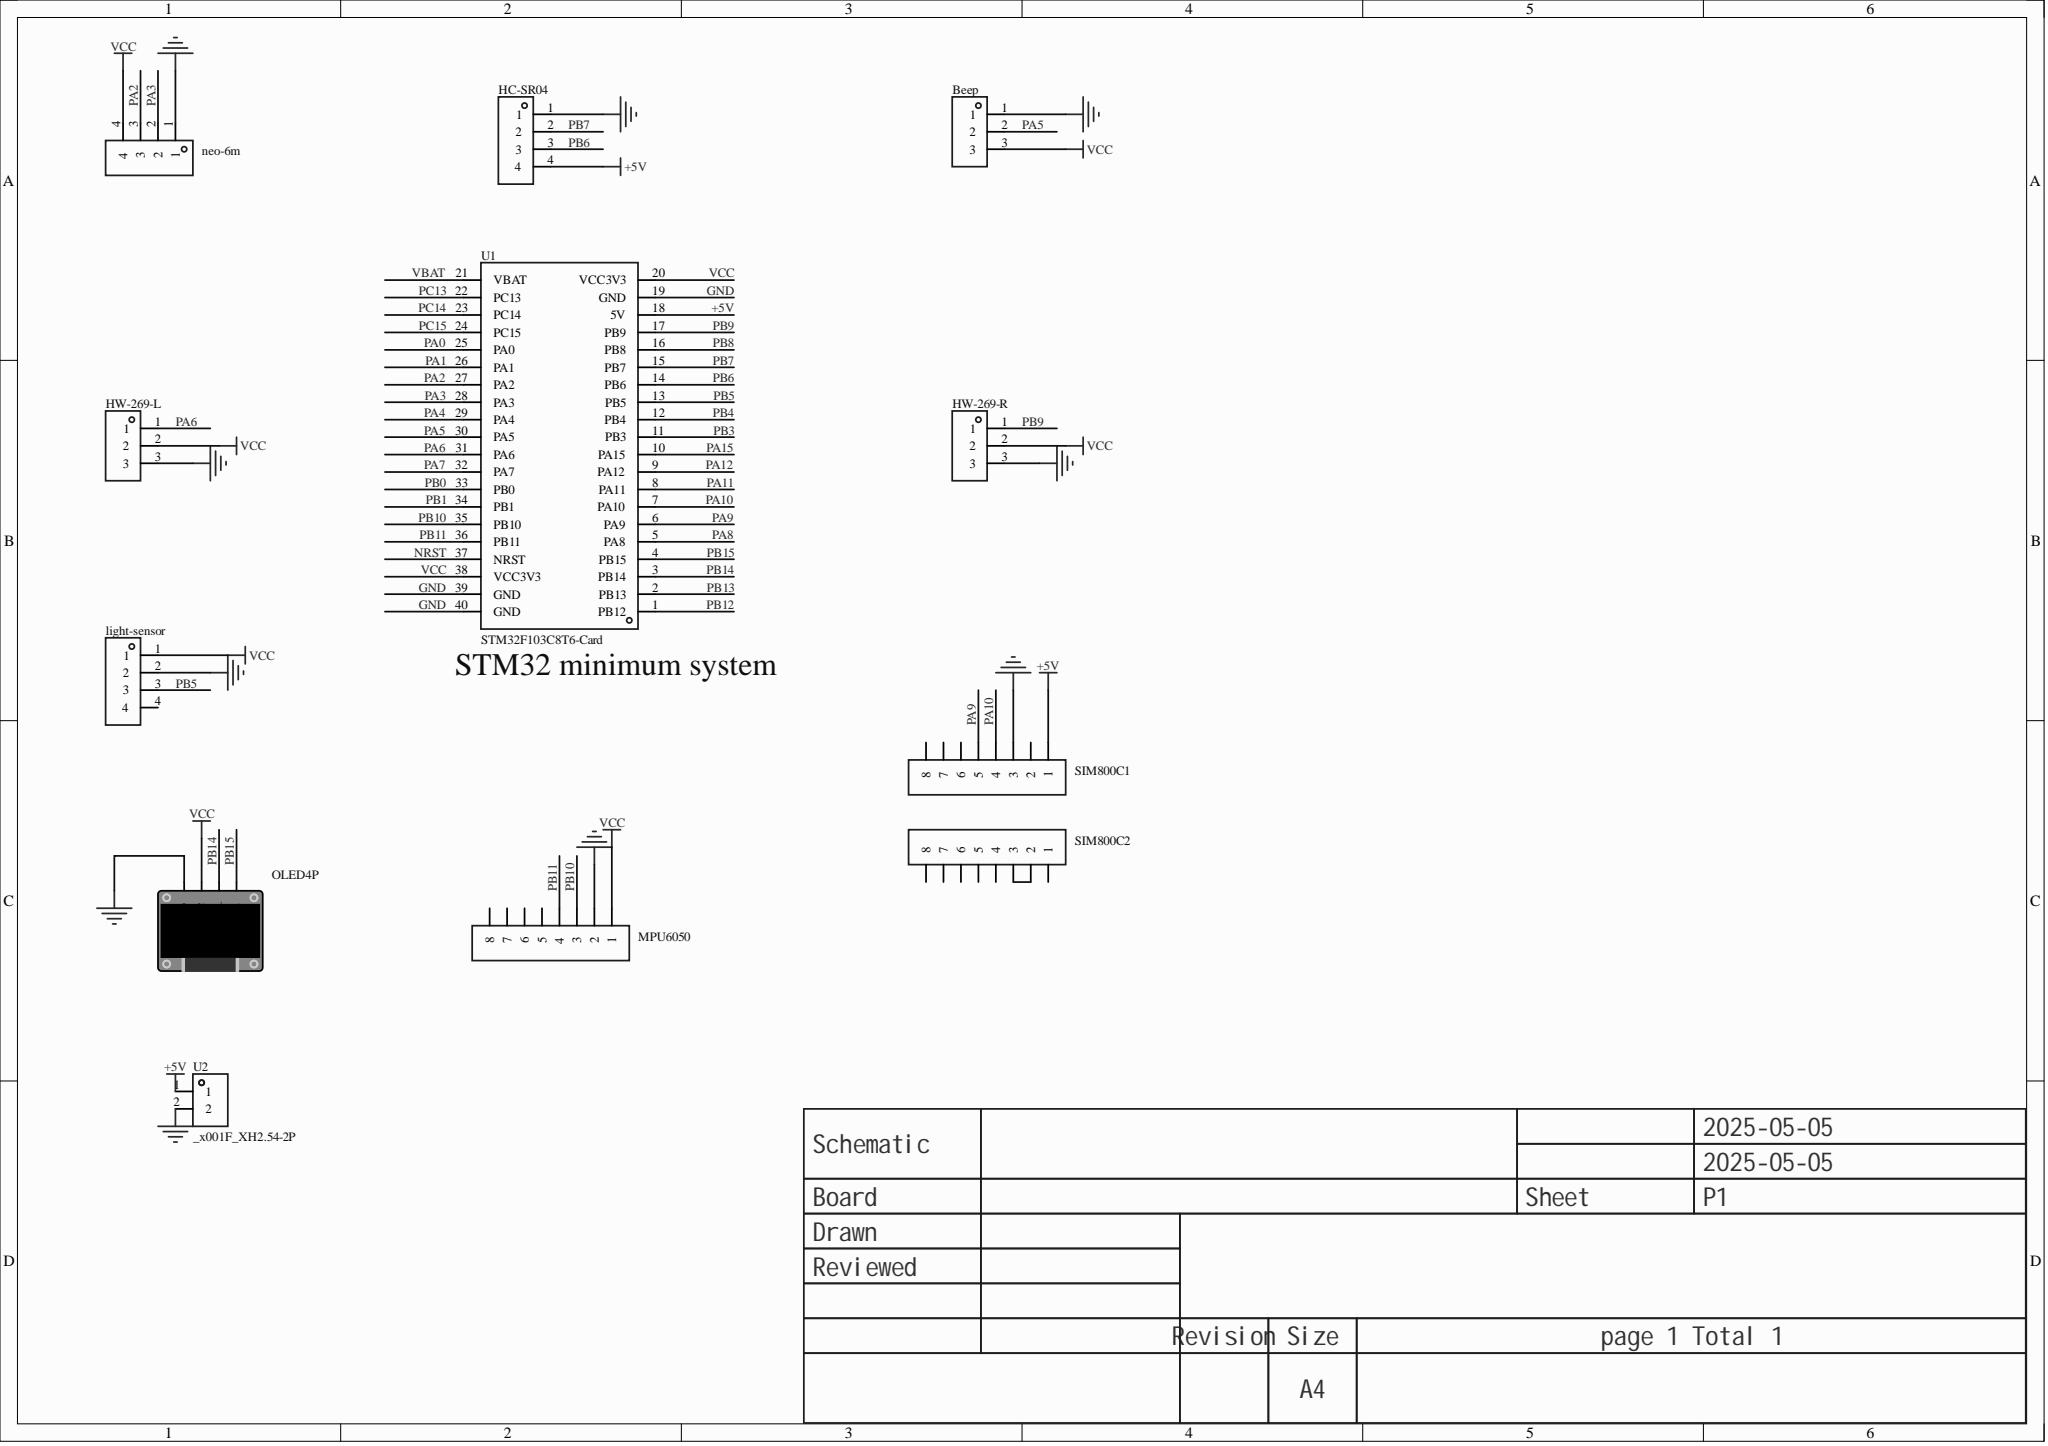Circuit board | Altium Designer | 12 parts | 18 nets
Bill of materials:
Comment,Description,Designator,Footprint,LibRef,Quantity
"","","Beep, HW-269-L, HW-269-R","HDR-TH_3P-P2.54-V-F","HDR-F_2.54_1x3P","3"
"","","HC-SR04, light-sensor, neo-6m","HDR-TH_4P-P2.54-V-F","HDR-F_2.54_1x4P","3"
"","","MPU6050, SIM800C1, SIM800C2","HDR-TH_8P-P2.54-V-F-1","HDR-F_2.54_1x8P","3"
"","","OLED4P","0.96OLED_4P","0.96OLED模块_4P","1"
"STM32F103C8T6-Card","","U1","CONN-TH_L53.3-W22.9_STM32F103C8T6-CARD","STM32F103C8T6-Card","1"
"_x001F_XH2.54-2P","","U2","CONN-TH_2P-P2.54-V","_x001F_XH2.54-2P","1"
Netlist (Protel format):
[
Beep
HDR-TH_3P-P2.54-V-F




]
[
HC-SR04
HDR-TH_4P-P2.54-V-F




]
[
HW-269-L
HDR-TH_3P-P2.54-V-F




]
[
HW-269-R
HDR-TH_3P-P2.54-V-F




]
[
light-sensor
HDR-TH_4P-P2.54-V-F




]
[
MPU6050
HDR-TH_8P-P2.54-V-F-1




]
[
neo-6m
HDR-TH_4P-P2.54-V-F




]
[
OLED4P
0.96OLED_4P




]
[
SIM800C1
HDR-TH_8P-P2.54-V-F-1




]
[
SIM800C2
HDR-TH_8P-P2.54-V-F-1




]
[
U1
CONN-TH_L53.3-W22.9_STM32F103C8T6-CARD
STM32F103C8T6-Card



]
[
U2
CONN-TH_2P-P2.54-V
_x001F_XH2.54-2P



]
(
VCC
Beep-3
HW-269-L-2
HW-269-R-2
light-sensor-1
MPU6050-1
neo-6m-4
OLED4P-2
U1-20
U1-38
)
(
PB15
OLED4P-4
U1-4
)
(
PB14
OLED4P-3
U1-3
)
(
PB11
MPU6050-4
U1-36
)
(
PB10
MPU6050-3
U1-35
)
(
PB9
HW-269-R-1
U1-17
)
(
PB7
HC-SR04-2
U1-15
)
(
PB6
HC-SR04-3
U1-14
)
(
PB5
light-sensor-3
U1-13
)
(
PA10
SIM800C1-4
U1-7
)
(
PA9
SIM800C1-5
U1-6
)
(
PA6
HW-269-L-1
U1-31
)
(
PA5
Beep-2
U1-30
)
(
PA3
neo-6m-2
U1-28
)
(
PA2
neo-6m-3
U1-27
)
(
NetSIM800C2_2
SIM800C2-2
SIM800C2-3
)
(
GND
Beep-1
HC-SR04-1
HW-269-L-3
HW-269-R-3
light-sensor-2
MPU6050-2
neo-6m-1
OLED4P-1
SIM800C1-3
U1-19
U1-39
U1-40
U2-2
)
(
+5V
HC-SR04-4
SIM800C1-1
U1-18
U2-1
)